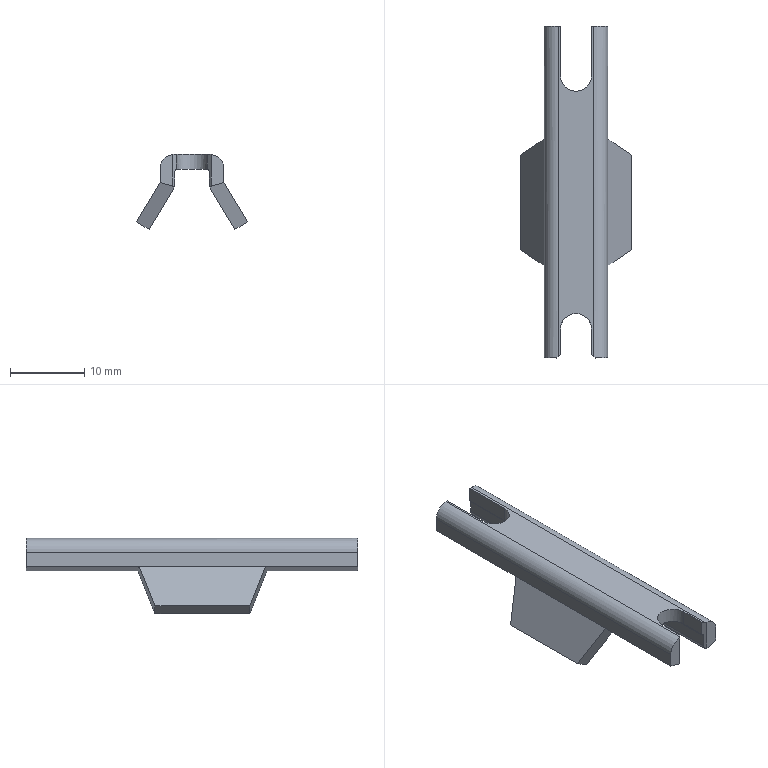Part | STEP file | Y300T_Y3035DB Front Plate_3 | 1 solid | 38 faces | box 14.986 x 44.8 x 10.145 mm | volume 1347 mm3 | plane 30 | cylinder 8 | commonest cylinder face diameters 0.6 x2 3.2 x2 3.8 x2 4.2 x2
STEP:
#1=CARTESIAN_POINT('',(-2.1,23.8,-2.017));
#2=VERTEX_POINT('',#1);
#3=CARTESIAN_POINT('',(-2.1,23.8,0.));
#4=VERTEX_POINT('',#3);
#5=CARTESIAN_POINT('',(-2.1,23.8,-10.145));
#6=DIRECTION('',(0.,0.,1.));
#7=VECTOR('',#6,1000.);
#8=LINE('',#5,#7);
#9=EDGE_CURVE('',#2,#4,#8,.T.);
#10=ORIENTED_EDGE('',*,*,#9,.F.);
#11=CARTESIAN_POINT('',(-2.3,23.8,-2.3));
#12=VERTEX_POINT('',#11);
#13=CARTESIAN_POINT('',(-2.,23.8,-2.3));
#14=DIRECTION('',(0.,1.,0.));
#15=DIRECTION('',(0.,0.,1.));
#16=AXIS2_PLACEMENT_3D('',#13,#14,#15);
#17=CIRCLE('',#16,0.3);
#18=EDGE_CURVE('',#12,#2,#17,.T.);
#19=ORIENTED_EDGE('',*,*,#18,.F.);
#20=CARTESIAN_POINT('',(-2.3,23.8,-3.911));
#21=VERTEX_POINT('',#20);
#22=CARTESIAN_POINT('',(-2.3,23.8,-4.355));
#23=DIRECTION('',(0.,0.,1.));
#24=VECTOR('',#23,1000.);
#25=LINE('',#22,#24);
#26=EDGE_CURVE('',#21,#12,#25,.T.);
#27=ORIENTED_EDGE('',*,*,#26,.F.);
#28=CARTESIAN_POINT('',(-2.363,23.8,-4.355));
#29=VERTEX_POINT('',#28);
#30=CARTESIAN_POINT('',(-3.9,23.8,-3.911));
#31=DIRECTION('',(0.,-1.,0.));
#32=DIRECTION('',(0.,0.,1.));
#33=AXIS2_PLACEMENT_3D('',#30,#31,#32);
#34=CIRCLE('',#33,1.6);
#35=EDGE_CURVE('',#29,#21,#34,.T.);
#36=ORIENTED_EDGE('',*,*,#35,.F.);
#37=CARTESIAN_POINT('',(-4.3,23.8,-3.8));
#38=VERTEX_POINT('',#37);
#39=CARTESIAN_POINT('',(-1.334,23.8,-4.651));
#40=DIRECTION('',(0.9613,0.,-0.2756));
#41=VECTOR('',#40,1000.);
#42=LINE('',#39,#41);
#43=EDGE_CURVE('',#38,#29,#42,.T.);
#44=ORIENTED_EDGE('',*,*,#43,.F.);
#45=CARTESIAN_POINT('',(-4.3,23.8,-1.9));
#46=VERTEX_POINT('',#45);
#47=CARTESIAN_POINT('',(-4.3,23.8,0.));
#48=DIRECTION('',(0.,0.,-1.));
#49=VECTOR('',#48,1000.);
#50=LINE('',#47,#49);
#51=EDGE_CURVE('',#46,#38,#50,.T.);
#52=ORIENTED_EDGE('',*,*,#51,.F.);
#53=CARTESIAN_POINT('',(-2.4,23.8,0.));
#54=VERTEX_POINT('',#53);
#55=CARTESIAN_POINT('',(-2.4,23.8,-1.9));
#56=DIRECTION('',(0.,-1.,0.));
#57=DIRECTION('',(0.,0.,1.));
#58=AXIS2_PLACEMENT_3D('',#55,#56,#57);
#59=CIRCLE('',#58,1.9);
#60=EDGE_CURVE('',#54,#46,#59,.T.);
#61=ORIENTED_EDGE('',*,*,#60,.F.);
#62=CARTESIAN_POINT('',(0.,23.8,0.));
#63=DIRECTION('',(1.,0.,0.));
#64=VECTOR('',#63,1000.);
#65=LINE('',#62,#64);
#66=EDGE_CURVE('',#54,#4,#65,.T.);
#67=ORIENTED_EDGE('',*,*,#66,.T.);
#68=EDGE_LOOP('',(#10,#19,#27,#36,#44,#52,#61,#67));
#69=FACE_OUTER_BOUND('',#68,.T.);
#70=CARTESIAN_POINT('',(0.,23.8,0.));
#71=DIRECTION('',(0.,1.,0.));
#72=DIRECTION('',(0.,0.,1.));
#73=AXIS2_PLACEMENT_3D('',#70,#71,#72);
#74=PLANE('',#73);
#75=ADVANCED_FACE('',(#69),#74,.T.);
#76=CARTESIAN_POINT('',(-4.3,-21.,-3.8));
#77=VERTEX_POINT('',#76);
#78=CARTESIAN_POINT('',(-2.6,-21.,-4.287));
#79=VERTEX_POINT('',#78);
#80=CARTESIAN_POINT('',(-4.3,-21.,-3.8));
#81=DIRECTION('',(0.9613,0.,-0.2756));
#82=VECTOR('',#81,1000.);
#83=LINE('',#80,#82);
#84=EDGE_CURVE('',#77,#79,#83,.T.);
#85=ORIENTED_EDGE('',*,*,#84,.T.);
#86=CARTESIAN_POINT('',(-2.6,-21.,-0.01056));
#87=VERTEX_POINT('',#86);
#88=CARTESIAN_POINT('',(-2.6,-21.,68.405));
#89=DIRECTION('',(0.,0.,1.));
#90=VECTOR('',#89,1000.);
#91=LINE('',#88,#90);
#92=EDGE_CURVE('',#79,#87,#91,.T.);
#93=ORIENTED_EDGE('',*,*,#92,.T.);
#94=CARTESIAN_POINT('',(-4.3,-21.,-1.9));
#95=VERTEX_POINT('',#94);
#96=CARTESIAN_POINT('',(-2.4,-21.,-1.9));
#97=DIRECTION('',(0.,-1.,0.));
#98=DIRECTION('',(0.,0.,1.));
#99=AXIS2_PLACEMENT_3D('',#96,#97,#98);
#100=CIRCLE('',#99,1.9);
#101=EDGE_CURVE('',#87,#95,#100,.T.);
#102=ORIENTED_EDGE('',*,*,#101,.T.);
#103=CARTESIAN_POINT('',(-4.3,-21.,0.));
#104=DIRECTION('',(0.,0.,1.));
#105=VECTOR('',#104,1000.);
#106=LINE('',#103,#105);
#107=EDGE_CURVE('',#77,#95,#106,.T.);
#108=ORIENTED_EDGE('',*,*,#107,.F.);
#109=EDGE_LOOP('',(#85,#93,#102,#108));
#110=FACE_OUTER_BOUND('',#109,.T.);
#111=CARTESIAN_POINT('',(-7.493,-21.,68.405));
#112=DIRECTION('',(0.,1.,0.));
#113=DIRECTION('',(0.,0.,1.));
#114=AXIS2_PLACEMENT_3D('',#111,#112,#113);
#115=PLANE('',#114);
#116=ADVANCED_FACE('',(#110),#115,.F.);
#117=CARTESIAN_POINT('',(7.493,6.4,-9.114));
#118=VERTEX_POINT('',#117);
#119=CARTESIAN_POINT('',(4.3,8.535,-3.8));
#120=VERTEX_POINT('',#119);
#121=CARTESIAN_POINT('',(7.493,6.4,-9.114));
#122=DIRECTION('',(-0.487,0.3256,0.8105));
#123=VECTOR('',#122,1000.);
#124=LINE('',#121,#123);
#125=EDGE_CURVE('',#118,#120,#124,.T.);
#126=ORIENTED_EDGE('',*,*,#125,.T.);
#127=CARTESIAN_POINT('',(4.3,-8.535,-3.8));
#128=VERTEX_POINT('',#127);
#129=CARTESIAN_POINT('',(4.3,23.8,-3.8));
#130=DIRECTION('',(0.,-1.,0.));
#131=VECTOR('',#130,1000.);
#132=LINE('',#129,#131);
#133=EDGE_CURVE('',#120,#128,#132,.T.);
#134=ORIENTED_EDGE('',*,*,#133,.T.);
#135=CARTESIAN_POINT('',(7.493,-6.4,-9.114));
#136=VERTEX_POINT('',#135);
#137=CARTESIAN_POINT('',(7.493,-6.4,-9.114));
#138=DIRECTION('',(-0.487,-0.3256,0.8105));
#139=VECTOR('',#138,1000.);
#140=LINE('',#137,#139);
#141=EDGE_CURVE('',#136,#128,#140,.T.);
#142=ORIENTED_EDGE('',*,*,#141,.F.);
#143=CARTESIAN_POINT('',(7.493,23.8,-9.114));
#144=DIRECTION('',(0.,-1.,0.));
#145=VECTOR('',#144,1000.);
#146=LINE('',#143,#145);
#147=EDGE_CURVE('',#118,#136,#146,.T.);
#148=ORIENTED_EDGE('',*,*,#147,.F.);
#149=EDGE_LOOP('',(#126,#134,#142,#148));
#150=FACE_OUTER_BOUND('',#149,.T.);
#151=CARTESIAN_POINT('',(4.3,23.8,-3.8));
#152=DIRECTION('',(-0.8572,0.,-0.515));
#153=DIRECTION('',(-0.515,0.,0.8572));
#154=AXIS2_PLACEMENT_3D('',#151,#152,#153);
#155=PLANE('',#154);
#156=ADVANCED_FACE('',(#150),#155,.F.);
#157=CARTESIAN_POINT('',(5.779,6.4,-10.145));
#158=VERTEX_POINT('',#157);
#159=CARTESIAN_POINT('',(-13.936,6.4,-21.99));
#160=DIRECTION('',(0.8572,0.,0.515));
#161=VECTOR('',#160,1000.);
#162=LINE('',#159,#161);
#163=EDGE_CURVE('',#158,#118,#162,.T.);
#164=ORIENTED_EDGE('',*,*,#163,.T.);
#165=ORIENTED_EDGE('',*,*,#147,.T.);
#166=CARTESIAN_POINT('',(5.779,-6.4,-10.145));
#167=VERTEX_POINT('',#166);
#168=CARTESIAN_POINT('',(-13.936,-6.4,-21.99));
#169=DIRECTION('',(0.8572,0.,0.515));
#170=VECTOR('',#169,1000.);
#171=LINE('',#168,#170);
#172=EDGE_CURVE('',#167,#136,#171,.T.);
#173=ORIENTED_EDGE('',*,*,#172,.F.);
#174=CARTESIAN_POINT('',(5.779,23.8,-10.145));
#175=DIRECTION('',(0.,-1.,0.));
#176=VECTOR('',#175,1000.);
#177=LINE('',#174,#176);
#178=EDGE_CURVE('',#158,#167,#177,.T.);
#179=ORIENTED_EDGE('',*,*,#178,.F.);
#180=EDGE_LOOP('',(#164,#165,#173,#179));
#181=FACE_OUTER_BOUND('',#180,.T.);
#182=CARTESIAN_POINT('',(7.493,23.8,-9.114));
#183=DIRECTION('',(-0.515,0.,0.8572));
#184=DIRECTION('',(0.8572,0.,0.515));
#185=AXIS2_PLACEMENT_3D('',#182,#183,#184);
#186=PLANE('',#185);
#187=ADVANCED_FACE('',(#181),#186,.F.);
#188=ORIENTED_EDGE('',*,*,#178,.T.);
#189=CARTESIAN_POINT('',(2.529,-8.573,-4.735));
#190=VERTEX_POINT('',#189);
#191=CARTESIAN_POINT('',(5.779,-6.4,-10.145));
#192=DIRECTION('',(0.487,0.3256,-0.8105));
#193=VECTOR('',#192,1000.);
#194=LINE('',#191,#193);
#195=EDGE_CURVE('',#190,#167,#194,.T.);
#196=ORIENTED_EDGE('',*,*,#195,.F.);
#197=CARTESIAN_POINT('',(2.529,8.573,-4.735));
#198=VERTEX_POINT('',#197);
#199=CARTESIAN_POINT('',(2.529,23.8,-4.735));
#200=DIRECTION('',(0.,1.,0.));
#201=VECTOR('',#200,1000.);
#202=LINE('',#199,#201);
#203=EDGE_CURVE('',#190,#198,#202,.T.);
#204=ORIENTED_EDGE('',*,*,#203,.T.);
#205=CARTESIAN_POINT('',(5.779,6.4,-10.145));
#206=DIRECTION('',(0.487,-0.3256,-0.8105));
#207=VECTOR('',#206,1000.);
#208=LINE('',#205,#207);
#209=EDGE_CURVE('',#198,#158,#208,.T.);
#210=ORIENTED_EDGE('',*,*,#209,.T.);
#211=EDGE_LOOP('',(#188,#196,#204,#210));
#212=FACE_OUTER_BOUND('',#211,.T.);
#213=CARTESIAN_POINT('',(5.779,23.8,-10.145));
#214=DIRECTION('',(0.8572,0.,0.515));
#215=DIRECTION('',(0.515,0.,-0.8572));
#216=AXIS2_PLACEMENT_3D('',#213,#214,#215);
#217=PLANE('',#216);
#218=ADVANCED_FACE('',(#212),#217,.F.);
#219=CARTESIAN_POINT('',(2.1,23.8,-2.017));
#220=VERTEX_POINT('',#219);
#221=CARTESIAN_POINT('',(2.1,23.8,0.));
#222=VERTEX_POINT('',#221);
#223=CARTESIAN_POINT('',(2.1,23.8,-10.145));
#224=DIRECTION('',(0.,0.,1.));
#225=VECTOR('',#224,1000.);
#226=LINE('',#223,#225);
#227=EDGE_CURVE('',#220,#222,#226,.T.);
#228=ORIENTED_EDGE('',*,*,#227,.T.);
#229=CARTESIAN_POINT('',(2.4,23.8,0.));
#230=VERTEX_POINT('',#229);
#231=CARTESIAN_POINT('',(0.,23.8,0.));
#232=DIRECTION('',(1.,0.,0.));
#233=VECTOR('',#232,1000.);
#234=LINE('',#231,#233);
#235=EDGE_CURVE('',#222,#230,#234,.T.);
#236=ORIENTED_EDGE('',*,*,#235,.T.);
#237=CARTESIAN_POINT('',(4.3,23.8,-1.9));
#238=VERTEX_POINT('',#237);
#239=CARTESIAN_POINT('',(2.4,23.8,-1.9));
#240=DIRECTION('',(0.,1.,0.));
#241=DIRECTION('',(0.,0.,1.));
#242=AXIS2_PLACEMENT_3D('',#239,#240,#241);
#243=CIRCLE('',#242,1.9);
#244=EDGE_CURVE('',#230,#238,#243,.T.);
#245=ORIENTED_EDGE('',*,*,#244,.T.);
#246=CARTESIAN_POINT('',(4.3,23.8,-3.8));
#247=VERTEX_POINT('',#246);
#248=CARTESIAN_POINT('',(4.3,23.8,0.));
#249=DIRECTION('',(0.,0.,-1.));
#250=VECTOR('',#249,1000.);
#251=LINE('',#248,#250);
#252=EDGE_CURVE('',#238,#247,#251,.T.);
#253=ORIENTED_EDGE('',*,*,#252,.T.);
#254=CARTESIAN_POINT('',(2.363,23.8,-4.355));
#255=VERTEX_POINT('',#254);
#256=CARTESIAN_POINT('',(1.334,23.8,-4.651));
#257=DIRECTION('',(-0.9613,0.,-0.2756));
#258=VECTOR('',#257,1000.);
#259=LINE('',#256,#258);
#260=EDGE_CURVE('',#247,#255,#259,.T.);
#261=ORIENTED_EDGE('',*,*,#260,.T.);
#262=CARTESIAN_POINT('',(2.3,23.8,-3.911));
#263=VERTEX_POINT('',#262);
#264=CARTESIAN_POINT('',(3.9,23.8,-3.911));
#265=DIRECTION('',(0.,1.,0.));
#266=DIRECTION('',(0.,0.,1.));
#267=AXIS2_PLACEMENT_3D('',#264,#265,#266);
#268=CIRCLE('',#267,1.6);
#269=EDGE_CURVE('',#255,#263,#268,.T.);
#270=ORIENTED_EDGE('',*,*,#269,.T.);
#271=CARTESIAN_POINT('',(2.3,23.8,-2.3));
#272=VERTEX_POINT('',#271);
#273=CARTESIAN_POINT('',(2.3,23.8,-4.355));
#274=DIRECTION('',(0.,0.,1.));
#275=VECTOR('',#274,1000.);
#276=LINE('',#273,#275);
#277=EDGE_CURVE('',#263,#272,#276,.T.);
#278=ORIENTED_EDGE('',*,*,#277,.T.);
#279=CARTESIAN_POINT('',(2.,23.8,-2.3));
#280=DIRECTION('',(0.,-1.,0.));
#281=DIRECTION('',(0.,0.,1.));
#282=AXIS2_PLACEMENT_3D('',#279,#280,#281);
#283=CIRCLE('',#282,0.3);
#284=EDGE_CURVE('',#272,#220,#283,.T.);
#285=ORIENTED_EDGE('',*,*,#284,.T.);
#286=EDGE_LOOP('',(#228,#236,#245,#253,#261,#270,#278,#285));
#287=FACE_OUTER_BOUND('',#286,.T.);
#288=CARTESIAN_POINT('',(0.,23.8,0.));
#289=DIRECTION('',(0.,1.,0.));
#290=DIRECTION('',(0.,0.,1.));
#291=AXIS2_PLACEMENT_3D('',#288,#289,#290);
#292=PLANE('',#291);
#293=ADVANCED_FACE('',(#287),#292,.T.);
#294=CARTESIAN_POINT('',(-2.4,-20.8,0.));
#295=VERTEX_POINT('',#294);
#296=CARTESIAN_POINT('',(-2.4,23.8,0.));
#297=DIRECTION('',(0.,1.,0.));
#298=VECTOR('',#297,1000.);
#299=LINE('',#296,#298);
#300=EDGE_CURVE('',#295,#54,#299,.T.);
#301=ORIENTED_EDGE('',*,*,#300,.F.);
#302=CARTESIAN_POINT('',(-2.1,-20.5,0.));
#303=VERTEX_POINT('',#302);
#304=CARTESIAN_POINT('',(-2.6,-21.,0.));
#305=DIRECTION('',(0.7071,0.7071,0.));
#306=VECTOR('',#305,1000.);
#307=LINE('',#304,#306);
#308=EDGE_CURVE('',#295,#303,#307,.T.);
#309=ORIENTED_EDGE('',*,*,#308,.T.);
#310=CARTESIAN_POINT('',(-2.1,-17.1,0.));
#311=VERTEX_POINT('',#310);
#312=CARTESIAN_POINT('',(-2.1,-21.,0.));
#313=DIRECTION('',(0.,-1.,0.));
#314=VECTOR('',#313,1000.);
#315=LINE('',#312,#314);
#316=EDGE_CURVE('',#311,#303,#315,.T.);
#317=ORIENTED_EDGE('',*,*,#316,.F.);
#318=CARTESIAN_POINT('',(2.1,-17.1,0.));
#319=VERTEX_POINT('',#318);
#320=CARTESIAN_POINT('',(0.,-17.1,0.));
#321=DIRECTION('',(0.,0.,1.));
#322=DIRECTION('',(-1.,0.,0.));
#323=AXIS2_PLACEMENT_3D('',#320,#321,#322);
#324=CIRCLE('',#323,2.1);
#325=EDGE_CURVE('',#319,#311,#324,.T.);
#326=ORIENTED_EDGE('',*,*,#325,.F.);
#327=CARTESIAN_POINT('',(2.1,-20.5,0.));
#328=VERTEX_POINT('',#327);
#329=CARTESIAN_POINT('',(2.1,-21.,0.));
#330=DIRECTION('',(0.,1.,0.));
#331=VECTOR('',#330,1000.);
#332=LINE('',#329,#331);
#333=EDGE_CURVE('',#328,#319,#332,.T.);
#334=ORIENTED_EDGE('',*,*,#333,.F.);
#335=CARTESIAN_POINT('',(2.4,-20.8,0.));
#336=VERTEX_POINT('',#335);
#337=CARTESIAN_POINT('',(2.6,-21.,0.));
#338=DIRECTION('',(0.7071,-0.7071,0.));
#339=VECTOR('',#338,1000.);
#340=LINE('',#337,#339);
#341=EDGE_CURVE('',#328,#336,#340,.T.);
#342=ORIENTED_EDGE('',*,*,#341,.T.);
#343=CARTESIAN_POINT('',(2.4,23.8,0.));
#344=DIRECTION('',(0.,1.,0.));
#345=VECTOR('',#344,1000.);
#346=LINE('',#343,#345);
#347=EDGE_CURVE('',#336,#230,#346,.T.);
#348=ORIENTED_EDGE('',*,*,#347,.T.);
#349=ORIENTED_EDGE('',*,*,#235,.F.);
#350=CARTESIAN_POINT('',(2.1,17.1,0.));
#351=VERTEX_POINT('',#350);
#352=CARTESIAN_POINT('',(2.1,23.8,0.));
#353=DIRECTION('',(0.,1.,0.));
#354=VECTOR('',#353,1000.);
#355=LINE('',#352,#354);
#356=EDGE_CURVE('',#351,#222,#355,.T.);
#357=ORIENTED_EDGE('',*,*,#356,.F.);
#358=CARTESIAN_POINT('',(-2.1,17.1,0.));
#359=VERTEX_POINT('',#358);
#360=CARTESIAN_POINT('',(0.,17.1,0.));
#361=DIRECTION('',(0.,0.,1.));
#362=DIRECTION('',(1.,0.,0.));
#363=AXIS2_PLACEMENT_3D('',#360,#361,#362);
#364=CIRCLE('',#363,2.1);
#365=EDGE_CURVE('',#359,#351,#364,.T.);
#366=ORIENTED_EDGE('',*,*,#365,.F.);
#367=CARTESIAN_POINT('',(-2.1,23.8,0.));
#368=DIRECTION('',(0.,-1.,0.));
#369=VECTOR('',#368,1000.);
#370=LINE('',#367,#369);
#371=EDGE_CURVE('',#4,#359,#370,.T.);
#372=ORIENTED_EDGE('',*,*,#371,.F.);
#373=ORIENTED_EDGE('',*,*,#66,.F.);
#374=EDGE_LOOP('',(#301,#309,#317,#326,#334,#342,#348,#349,#357,#366,#372,#373));
#375=FACE_OUTER_BOUND('',#374,.T.);
#376=CARTESIAN_POINT('',(0.,23.8,0.));
#377=DIRECTION('',(0.,0.,-1.));
#378=DIRECTION('',(-1.,0.,0.));
#379=AXIS2_PLACEMENT_3D('',#376,#377,#378);
#380=PLANE('',#379);
#381=ADVANCED_FACE('',(#375),#380,.F.);
#382=CARTESIAN_POINT('',(4.3,-21.,-1.9));
#383=VERTEX_POINT('',#382);
#384=CARTESIAN_POINT('',(4.3,23.8,-1.9));
#385=DIRECTION('',(0.,-1.,0.));
#386=VECTOR('',#385,1000.);
#387=LINE('',#384,#386);
#388=EDGE_CURVE('',#238,#383,#387,.T.);
#389=ORIENTED_EDGE('',*,*,#388,.T.);
#390=CARTESIAN_POINT('',(4.3,-21.,-3.8));
#391=VERTEX_POINT('',#390);
#392=CARTESIAN_POINT('',(4.3,-21.,0.));
#393=DIRECTION('',(0.,0.,-1.));
#394=VECTOR('',#393,1000.);
#395=LINE('',#392,#394);
#396=EDGE_CURVE('',#383,#391,#395,.T.);
#397=ORIENTED_EDGE('',*,*,#396,.T.);
#398=CARTESIAN_POINT('',(4.3,-23.8,-3.8));
#399=DIRECTION('',(0.,1.,0.));
#400=VECTOR('',#399,1000.);
#401=LINE('',#398,#400);
#402=EDGE_CURVE('',#391,#128,#401,.T.);
#403=ORIENTED_EDGE('',*,*,#402,.T.);
#404=ORIENTED_EDGE('',*,*,#133,.F.);
#405=CARTESIAN_POINT('',(4.3,23.8,-3.8));
#406=DIRECTION('',(0.,-1.,0.));
#407=VECTOR('',#406,1000.);
#408=LINE('',#405,#407);
#409=EDGE_CURVE('',#247,#120,#408,.T.);
#410=ORIENTED_EDGE('',*,*,#409,.F.);
#411=ORIENTED_EDGE('',*,*,#252,.F.);
#412=EDGE_LOOP('',(#389,#397,#403,#404,#410,#411));
#413=FACE_OUTER_BOUND('',#412,.T.);
#414=CARTESIAN_POINT('',(4.3,23.8,0.));
#415=DIRECTION('',(-1.,0.,0.));
#416=DIRECTION('',(0.,0.,1.));
#417=AXIS2_PLACEMENT_3D('',#414,#415,#416);
#418=PLANE('',#417);
#419=ADVANCED_FACE('',(#413),#418,.F.);
#420=CARTESIAN_POINT('',(2.3,-20.7,-3.911));
#421=VERTEX_POINT('',#420);
#422=CARTESIAN_POINT('',(2.3,23.8,-3.911));
#423=DIRECTION('',(0.,-1.,0.));
#424=VECTOR('',#423,1000.);
#425=LINE('',#422,#424);
#426=EDGE_CURVE('',#263,#421,#425,.T.);
#427=ORIENTED_EDGE('',*,*,#426,.T.);
#428=CARTESIAN_POINT('',(2.3,-20.7,-2.3));
#429=VERTEX_POINT('',#428);
#430=CARTESIAN_POINT('',(2.3,-20.7,68.405));
#431=DIRECTION('',(0.,0.,1.));
#432=VECTOR('',#431,1000.);
#433=LINE('',#430,#432);
#434=EDGE_CURVE('',#421,#429,#433,.T.);
#435=ORIENTED_EDGE('',*,*,#434,.T.);
#436=CARTESIAN_POINT('',(2.3,23.8,-2.3));
#437=DIRECTION('',(0.,1.,0.));
#438=VECTOR('',#437,1000.);
#439=LINE('',#436,#438);
#440=EDGE_CURVE('',#429,#272,#439,.T.);
#441=ORIENTED_EDGE('',*,*,#440,.T.);
#442=ORIENTED_EDGE('',*,*,#277,.F.);
#443=EDGE_LOOP('',(#427,#435,#441,#442));
#444=FACE_OUTER_BOUND('',#443,.T.);
#445=CARTESIAN_POINT('',(2.3,23.8,-4.355));
#446=DIRECTION('',(1.,0.,0.));
#447=DIRECTION('',(0.,0.,-1.));
#448=AXIS2_PLACEMENT_3D('',#445,#446,#447);
#449=PLANE('',#448);
#450=ADVANCED_FACE('',(#444),#449,.F.);
#451=CARTESIAN_POINT('',(-2.,16.46,-2.));
#452=VERTEX_POINT('',#451);
#453=CARTESIAN_POINT('',(-2.,-16.46,-2.));
#454=VERTEX_POINT('',#453);
#455=CARTESIAN_POINT('',(-2.,0.,-2.));
#456=DIRECTION('',(0.,-1.,0.));
#457=VECTOR('',#456,1000.);
#458=LINE('',#455,#457);
#459=EDGE_CURVE('',#452,#454,#458,.T.);
#460=ORIENTED_EDGE('',*,*,#459,.F.);
#461=CARTESIAN_POINT('',(2.,16.46,-2.));
#462=VERTEX_POINT('',#461);
#463=CARTESIAN_POINT('',(0.,17.1,-2.));
#464=DIRECTION('',(0.,0.,1.));
#465=DIRECTION('',(1.,0.,0.));
#466=AXIS2_PLACEMENT_3D('',#463,#464,#465);
#467=CIRCLE('',#466,2.1);
#468=EDGE_CURVE('',#452,#462,#467,.T.);
#469=ORIENTED_EDGE('',*,*,#468,.T.);
#470=CARTESIAN_POINT('',(2.,-16.46,-2.));
#471=VERTEX_POINT('',#470);
#472=CARTESIAN_POINT('',(2.,0.,-2.));
#473=DIRECTION('',(0.,-1.,0.));
#474=VECTOR('',#473,1000.);
#475=LINE('',#472,#474);
#476=EDGE_CURVE('',#462,#471,#475,.T.);
#477=ORIENTED_EDGE('',*,*,#476,.T.);
#478=CARTESIAN_POINT('',(0.,-17.1,-2.));
#479=DIRECTION('',(0.,0.,1.));
#480=DIRECTION('',(1.,0.,0.));
#481=AXIS2_PLACEMENT_3D('',#478,#479,#480);
#482=CIRCLE('',#481,2.1);
#483=EDGE_CURVE('',#471,#454,#482,.T.);
#484=ORIENTED_EDGE('',*,*,#483,.T.);
#485=EDGE_LOOP('',(#460,#469,#477,#484));
#486=FACE_OUTER_BOUND('',#485,.T.);
#487=CARTESIAN_POINT('',(2.3,23.8,-2.));
#488=DIRECTION('',(0.,0.,1.));
#489=DIRECTION('',(1.,0.,0.));
#490=AXIS2_PLACEMENT_3D('',#487,#488,#489);
#491=PLANE('',#490);
#492=ADVANCED_FACE('',(#486),#491,.F.);
#493=ORIENTED_EDGE('',*,*,#209,.F.);
#494=CARTESIAN_POINT('',(2.363,8.714,-4.355));
#495=VERTEX_POINT('',#494);
#496=CARTESIAN_POINT('',(2.529,8.573,-4.735));
#497=CARTESIAN_POINT('',(2.457,8.621,-4.616));
#498=CARTESIAN_POINT('',(2.402,8.668,-4.489));
#499=CARTESIAN_POINT('',(2.363,8.714,-4.355));
#500=(BOUNDED_CURVE()B_SPLINE_CURVE(3,(#496,#497,#498,#499),.UNSPECIFIED.,.F.,.F.)B_SPLINE_CURVE_WITH_KNOTS((4,4),(1.571,1.83),.UNSPECIFIED.)CURVE()GEOMETRIC_REPRESENTATION_ITEM()RATIONAL_B_SPLINE_CURVE((1.,0.9944,0.9944,1.))REPRESENTATION_ITEM(''));
#501=EDGE_CURVE('',#198,#495,#500,.T.);
#502=ORIENTED_EDGE('',*,*,#501,.T.);
#503=CARTESIAN_POINT('',(-17.018,10.511,-9.913));
#504=DIRECTION('',(-0.9575,0.08877,-0.2745));
#505=VECTOR('',#504,1000.);
#506=LINE('',#503,#505);
#507=EDGE_CURVE('',#120,#495,#506,.T.);
#508=ORIENTED_EDGE('',*,*,#507,.F.);
#509=ORIENTED_EDGE('',*,*,#125,.F.);
#510=ORIENTED_EDGE('',*,*,#163,.F.);
#511=EDGE_LOOP('',(#493,#502,#508,#509,#510));
#512=FACE_OUTER_BOUND('',#511,.T.);
#513=CARTESIAN_POINT('',(-13.936,6.4,-21.99));
#514=DIRECTION('',(0.1677,0.9455,-0.2791));
#515=DIRECTION('',(0.,0.2831,0.9591));
#516=AXIS2_PLACEMENT_3D('',#513,#514,#515);
#517=PLANE('',#516);
#518=ADVANCED_FACE('',(#512),#517,.T.);
#519=ORIENTED_EDGE('',*,*,#507,.T.);
#520=CARTESIAN_POINT('',(2.363,8.714,-4.355));
#521=DIRECTION('',(0.,1.,0.));
#522=VECTOR('',#521,1000.);
#523=LINE('',#520,#522);
#524=EDGE_CURVE('',#495,#255,#523,.T.);
#525=ORIENTED_EDGE('',*,*,#524,.T.);
#526=ORIENTED_EDGE('',*,*,#260,.F.);
#527=ORIENTED_EDGE('',*,*,#409,.T.);
#528=EDGE_LOOP('',(#519,#525,#526,#527));
#529=FACE_OUTER_BOUND('',#528,.T.);
#530=CARTESIAN_POINT('',(4.3,0.,-3.8));
#531=DIRECTION('',(0.2756,0.,-0.9613));
#532=DIRECTION('',(-0.9613,0.,-0.2756));
#533=AXIS2_PLACEMENT_3D('',#530,#531,#532);
#534=PLANE('',#533);
#535=ADVANCED_FACE('',(#529),#534,.T.);
#536=ORIENTED_EDGE('',*,*,#347,.F.);
#537=CARTESIAN_POINT('',(2.6,-21.,-0.01056));
#538=VERTEX_POINT('',#537);
#539=CARTESIAN_POINT('',(2.4,-20.8,0.));
#540=CARTESIAN_POINT('',(2.467,-20.867,0.));
#541=CARTESIAN_POINT('',(2.534,-20.934,-0.003522));
#542=CARTESIAN_POINT('',(2.6,-21.,-0.01056));
#543=(BOUNDED_CURVE()B_SPLINE_CURVE(3,(#539,#540,#541,#542),.UNSPECIFIED.,.F.,.F.)B_SPLINE_CURVE_WITH_KNOTS((4,4),(4.712,4.818),.UNSPECIFIED.)CURVE()GEOMETRIC_REPRESENTATION_ITEM()RATIONAL_B_SPLINE_CURVE((1.,0.9991,0.9991,1.))REPRESENTATION_ITEM(''));
#544=EDGE_CURVE('',#336,#538,#543,.T.);
#545=ORIENTED_EDGE('',*,*,#544,.T.);
#546=CARTESIAN_POINT('',(2.4,-21.,-1.9));
#547=DIRECTION('',(0.,-1.,0.));
#548=DIRECTION('',(0.,0.,1.));
#549=AXIS2_PLACEMENT_3D('',#546,#547,#548);
#550=CIRCLE('',#549,1.9);
#551=EDGE_CURVE('',#383,#538,#550,.T.);
#552=ORIENTED_EDGE('',*,*,#551,.F.);
#553=ORIENTED_EDGE('',*,*,#388,.F.);
#554=ORIENTED_EDGE('',*,*,#244,.F.);
#555=EDGE_LOOP('',(#536,#545,#552,#553,#554));
#556=FACE_OUTER_BOUND('',#555,.T.);
#557=CARTESIAN_POINT('',(2.4,23.8,-1.9));
#558=DIRECTION('',(0.,-1.,0.));
#559=DIRECTION('',(0.,0.,-1.));
#560=AXIS2_PLACEMENT_3D('',#557,#558,#559);
#561=CYLINDRICAL_SURFACE('',#560,1.9);
#562=ADVANCED_FACE('',(#556),#561,.T.);
#563=ORIENTED_EDGE('',*,*,#440,.F.);
#564=CARTESIAN_POINT('',(2.1,-20.5,-2.017));
#565=VERTEX_POINT('',#564);
#566=CARTESIAN_POINT('',(2.3,-20.7,-2.3));
#567=CARTESIAN_POINT('',(2.3,-20.7,-2.168));
#568=CARTESIAN_POINT('',(2.224,-20.624,-2.061));
#569=CARTESIAN_POINT('',(2.1,-20.5,-2.017));
#570=(BOUNDED_CURVE()B_SPLINE_CURVE(3,(#566,#567,#568,#569),.UNSPECIFIED.,.F.,.F.)B_SPLINE_CURVE_WITH_KNOTS((4,4),(3.142,4.373),.UNSPECIFIED.)CURVE()GEOMETRIC_REPRESENTATION_ITEM()RATIONAL_B_SPLINE_CURVE((1.,0.8777,0.8777,1.))REPRESENTATION_ITEM(''));
#571=EDGE_CURVE('',#429,#565,#570,.T.);
#572=ORIENTED_EDGE('',*,*,#571,.T.);
#573=CARTESIAN_POINT('',(2.1,-17.1,-2.017));
#574=VERTEX_POINT('',#573);
#575=CARTESIAN_POINT('',(2.1,23.8,-2.017));
#576=DIRECTION('',(0.,1.,0.));
#577=VECTOR('',#576,1000.);
#578=LINE('',#575,#577);
#579=EDGE_CURVE('',#565,#574,#578,.T.);
#580=ORIENTED_EDGE('',*,*,#579,.T.);
#581=CARTESIAN_POINT('',(2.1,-17.1,-2.017));
#582=CARTESIAN_POINT('',(2.1,-16.882,-2.017));
#583=CARTESIAN_POINT('',(2.067,-16.667,-2.));
#584=CARTESIAN_POINT('',(2.,-16.46,-2.));
#585=B_SPLINE_CURVE_WITH_KNOTS('',3,(#581,#582,#583,#584),.UNSPECIFIED.,.F.,.F.,(4,4),(0.0006066,0.001255),.UNSPECIFIED.);
#586=EDGE_CURVE('',#574,#471,#585,.T.);
#587=ORIENTED_EDGE('',*,*,#586,.T.);
#588=ORIENTED_EDGE('',*,*,#476,.F.);
#589=CARTESIAN_POINT('',(2.1,17.1,-2.017));
#590=VERTEX_POINT('',#589);
#591=CARTESIAN_POINT('',(2.,16.46,-2.));
#592=CARTESIAN_POINT('',(2.033,16.564,-2.));
#593=CARTESIAN_POINT('',(2.058,16.67,-2.005));
#594=CARTESIAN_POINT('',(2.092,16.883,-2.014));
#595=CARTESIAN_POINT('',(2.1,16.991,-2.017));
#596=CARTESIAN_POINT('',(2.1,17.1,-2.017));
#597=B_SPLINE_CURVE_WITH_KNOTS('',3,(#591,#592,#593,#594,#595,#596),.UNSPECIFIED.,.F.,.F.,(4,2,4),(0.002836,0.003161,0.003485),.UNSPECIFIED.);
#598=EDGE_CURVE('',#462,#590,#597,.T.);
#599=ORIENTED_EDGE('',*,*,#598,.T.);
#600=CARTESIAN_POINT('',(2.1,23.8,-2.017));
#601=DIRECTION('',(0.,1.,0.));
#602=VECTOR('',#601,1000.);
#603=LINE('',#600,#602);
#604=EDGE_CURVE('',#590,#220,#603,.T.);
#605=ORIENTED_EDGE('',*,*,#604,.T.);
#606=ORIENTED_EDGE('',*,*,#284,.F.);
#607=EDGE_LOOP('',(#563,#572,#580,#587,#588,#599,#605,#606));
#608=FACE_OUTER_BOUND('',#607,.T.);
#609=CARTESIAN_POINT('',(2.,23.8,-2.3));
#610=DIRECTION('',(0.,1.,0.));
#611=DIRECTION('',(0.,0.,1.));
#612=AXIS2_PLACEMENT_3D('',#609,#610,#611);
#613=CYLINDRICAL_SURFACE('',#612,0.3);
#614=ADVANCED_FACE('',(#608),#613,.F.);
#615=CARTESIAN_POINT('',(2.363,-8.714,-4.355));
#616=VERTEX_POINT('',#615);
#617=CARTESIAN_POINT('',(2.363,-20.763,-4.355));
#618=VERTEX_POINT('',#617);
#619=CARTESIAN_POINT('',(2.363,-8.714,-4.355));
#620=DIRECTION('',(0.,-1.,0.));
#621=VECTOR('',#620,1000.);
#622=LINE('',#619,#621);
#623=EDGE_CURVE('',#616,#618,#622,.T.);
#624=ORIENTED_EDGE('',*,*,#623,.T.);
#625=CARTESIAN_POINT('',(2.363,-20.763,-4.355));
#626=CARTESIAN_POINT('',(2.321,-20.721,-4.211));
#627=CARTESIAN_POINT('',(2.3,-20.7,-4.062));
#628=CARTESIAN_POINT('',(2.3,-20.7,-3.911));
#629=(BOUNDED_CURVE()B_SPLINE_CURVE(3,(#625,#626,#627,#628),.UNSPECIFIED.,.F.,.F.)B_SPLINE_CURVE_WITH_KNOTS((4,4),(2.86,3.142),.UNSPECIFIED.)CURVE()GEOMETRIC_REPRESENTATION_ITEM()RATIONAL_B_SPLINE_CURVE((1.,0.9934,0.9934,1.))REPRESENTATION_ITEM(''));
#630=EDGE_CURVE('',#618,#421,#629,.T.);
#631=ORIENTED_EDGE('',*,*,#630,.T.);
#632=ORIENTED_EDGE('',*,*,#426,.F.);
#633=ORIENTED_EDGE('',*,*,#269,.F.);
#634=ORIENTED_EDGE('',*,*,#524,.F.);
#635=ORIENTED_EDGE('',*,*,#501,.F.);
#636=ORIENTED_EDGE('',*,*,#203,.F.);
#637=CARTESIAN_POINT('',(2.529,-8.573,-4.735));
#638=CARTESIAN_POINT('',(2.457,-8.621,-4.616));
#639=CARTESIAN_POINT('',(2.402,-8.668,-4.489));
#640=CARTESIAN_POINT('',(2.363,-8.714,-4.355));
#641=(BOUNDED_CURVE()B_SPLINE_CURVE(3,(#637,#638,#639,#640),.UNSPECIFIED.,.F.,.F.)B_SPLINE_CURVE_WITH_KNOTS((4,4),(1.571,1.83),.UNSPECIFIED.)CURVE()GEOMETRIC_REPRESENTATION_ITEM()RATIONAL_B_SPLINE_CURVE((1.,0.9944,0.9944,1.))REPRESENTATION_ITEM(''));
#642=EDGE_CURVE('',#190,#616,#641,.T.);
#643=ORIENTED_EDGE('',*,*,#642,.T.);
#644=EDGE_LOOP('',(#624,#631,#632,#633,#634,#635,#636,#643));
#645=FACE_OUTER_BOUND('',#644,.T.);
#646=CARTESIAN_POINT('',(3.9,23.8,-3.911));
#647=DIRECTION('',(0.,-1.,0.));
#648=DIRECTION('',(0.,0.,-1.));
#649=AXIS2_PLACEMENT_3D('',#646,#647,#648);
#650=CYLINDRICAL_SURFACE('',#649,1.6);
#651=ADVANCED_FACE('',(#645),#650,.T.);
#652=CARTESIAN_POINT('',(2.6,-21.,-4.287));
#653=VERTEX_POINT('',#652);
#654=CARTESIAN_POINT('',(4.3,-21.,-3.8));
#655=DIRECTION('',(0.9613,0.,0.2756));
#656=VECTOR('',#655,1000.);
#657=LINE('',#654,#656);
#658=EDGE_CURVE('',#653,#391,#657,.T.);
#659=ORIENTED_EDGE('',*,*,#658,.F.);
#660=CARTESIAN_POINT('',(-6.602,-11.798,-6.926));
#661=DIRECTION('',(-0.693,0.693,-0.1987));
#662=VECTOR('',#661,1000.);
#663=LINE('',#660,#662);
#664=EDGE_CURVE('',#653,#618,#663,.T.);
#665=ORIENTED_EDGE('',*,*,#664,.T.);
#666=ORIENTED_EDGE('',*,*,#623,.F.);
#667=CARTESIAN_POINT('',(-17.018,-10.511,-9.913));
#668=DIRECTION('',(-0.9575,-0.08877,-0.2745));
#669=VECTOR('',#668,1000.);
#670=LINE('',#667,#669);
#671=EDGE_CURVE('',#128,#616,#670,.T.);
#672=ORIENTED_EDGE('',*,*,#671,.F.);
#673=ORIENTED_EDGE('',*,*,#402,.F.);
#674=EDGE_LOOP('',(#659,#665,#666,#672,#673));
#675=FACE_OUTER_BOUND('',#674,.T.);
#676=CARTESIAN_POINT('',(4.3,0.,-3.8));
#677=DIRECTION('',(0.2756,0.,-0.9613));
#678=DIRECTION('',(-0.9613,0.,-0.2756));
#679=AXIS2_PLACEMENT_3D('',#676,#677,#678);
#680=PLANE('',#679);
#681=ADVANCED_FACE('',(#675),#680,.T.);
#682=ORIENTED_EDGE('',*,*,#195,.T.);
#683=ORIENTED_EDGE('',*,*,#172,.T.);
#684=ORIENTED_EDGE('',*,*,#141,.T.);
#685=ORIENTED_EDGE('',*,*,#671,.T.);
#686=ORIENTED_EDGE('',*,*,#642,.F.);
#687=EDGE_LOOP('',(#682,#683,#684,#685,#686));
#688=FACE_OUTER_BOUND('',#687,.T.);
#689=CARTESIAN_POINT('',(-13.936,-6.4,-21.99));
#690=DIRECTION('',(0.1677,-0.9455,-0.2791));
#691=DIRECTION('',(0.,-0.2831,0.9591));
#692=AXIS2_PLACEMENT_3D('',#689,#690,#691);
#693=PLANE('',#692);
#694=ADVANCED_FACE('',(#688),#693,.T.);
#695=CARTESIAN_POINT('',(-7.493,6.4,-9.114));
#696=VERTEX_POINT('',#695);
#697=CARTESIAN_POINT('',(-4.3,8.535,-3.8));
#698=VERTEX_POINT('',#697);
#699=CARTESIAN_POINT('',(-7.493,6.4,-9.114));
#700=DIRECTION('',(0.487,0.3256,0.8105));
#701=VECTOR('',#700,1000.);
#702=LINE('',#699,#701);
#703=EDGE_CURVE('',#696,#698,#702,.T.);
#704=ORIENTED_EDGE('',*,*,#703,.F.);
#705=CARTESIAN_POINT('',(-7.493,-6.4,-9.114));
#706=VERTEX_POINT('',#705);
#707=CARTESIAN_POINT('',(-7.493,23.8,-9.114));
#708=DIRECTION('',(0.,-1.,0.));
#709=VECTOR('',#708,1000.);
#710=LINE('',#707,#709);
#711=EDGE_CURVE('',#696,#706,#710,.T.);
#712=ORIENTED_EDGE('',*,*,#711,.T.);
#713=CARTESIAN_POINT('',(-4.3,-8.535,-3.8));
#714=VERTEX_POINT('',#713);
#715=CARTESIAN_POINT('',(-7.493,-6.4,-9.114));
#716=DIRECTION('',(0.487,-0.3256,0.8105));
#717=VECTOR('',#716,1000.);
#718=LINE('',#715,#717);
#719=EDGE_CURVE('',#706,#714,#718,.T.);
#720=ORIENTED_EDGE('',*,*,#719,.T.);
#721=CARTESIAN_POINT('',(-4.3,23.8,-3.8));
#722=DIRECTION('',(0.,-1.,0.));
#723=VECTOR('',#722,1000.);
#724=LINE('',#721,#723);
#725=EDGE_CURVE('',#698,#714,#724,.T.);
#726=ORIENTED_EDGE('',*,*,#725,.F.);
#727=EDGE_LOOP('',(#704,#712,#720,#726));
#728=FACE_OUTER_BOUND('',#727,.T.);
#729=CARTESIAN_POINT('',(-4.3,23.8,-3.8));
#730=DIRECTION('',(0.8572,0.,-0.515));
#731=DIRECTION('',(0.515,0.,0.8572));
#732=AXIS2_PLACEMENT_3D('',#729,#730,#731);
#733=PLANE('',#732);
#734=ADVANCED_FACE('',(#728),#733,.F.);
#735=CARTESIAN_POINT('',(-5.779,6.4,-10.145));
#736=VERTEX_POINT('',#735);
#737=CARTESIAN_POINT('',(13.936,6.4,-21.99));
#738=DIRECTION('',(-0.8572,0.,0.515));
#739=VECTOR('',#738,1000.);
#740=LINE('',#737,#739);
#741=EDGE_CURVE('',#736,#696,#740,.T.);
#742=ORIENTED_EDGE('',*,*,#741,.F.);
#743=CARTESIAN_POINT('',(-5.779,-6.4,-10.145));
#744=VERTEX_POINT('',#743);
#745=CARTESIAN_POINT('',(-5.779,23.8,-10.145));
#746=DIRECTION('',(0.,-1.,0.));
#747=VECTOR('',#746,1000.);
#748=LINE('',#745,#747);
#749=EDGE_CURVE('',#736,#744,#748,.T.);
#750=ORIENTED_EDGE('',*,*,#749,.T.);
#751=CARTESIAN_POINT('',(13.936,-6.4,-21.99));
#752=DIRECTION('',(-0.8572,0.,0.515));
#753=VECTOR('',#752,1000.);
#754=LINE('',#751,#753);
#755=EDGE_CURVE('',#744,#706,#754,.T.);
#756=ORIENTED_EDGE('',*,*,#755,.T.);
#757=ORIENTED_EDGE('',*,*,#711,.F.);
#758=EDGE_LOOP('',(#742,#750,#756,#757));
#759=FACE_OUTER_BOUND('',#758,.T.);
#760=CARTESIAN_POINT('',(-7.493,23.8,-9.114));
#761=DIRECTION('',(0.515,0.,0.8572));
#762=DIRECTION('',(-0.8572,0.,0.515));
#763=AXIS2_PLACEMENT_3D('',#760,#761,#762);
#764=PLANE('',#763);
#765=ADVANCED_FACE('',(#759),#764,.F.);
#766=ORIENTED_EDGE('',*,*,#749,.F.);
#767=CARTESIAN_POINT('',(-2.529,8.573,-4.735));
#768=VERTEX_POINT('',#767);
#769=CARTESIAN_POINT('',(-5.779,6.4,-10.145));
#770=DIRECTION('',(-0.487,-0.3256,-0.8105));
#771=VECTOR('',#770,1000.);
#772=LINE('',#769,#771);
#773=EDGE_CURVE('',#768,#736,#772,.T.);
#774=ORIENTED_EDGE('',*,*,#773,.F.);
#775=CARTESIAN_POINT('',(-2.529,-8.573,-4.735));
#776=VERTEX_POINT('',#775);
#777=CARTESIAN_POINT('',(-2.529,23.8,-4.735));
#778=DIRECTION('',(0.,1.,0.));
#779=VECTOR('',#778,1000.);
#780=LINE('',#777,#779);
#781=EDGE_CURVE('',#776,#768,#780,.T.);
#782=ORIENTED_EDGE('',*,*,#781,.F.);
#783=CARTESIAN_POINT('',(-5.779,-6.4,-10.145));
#784=DIRECTION('',(-0.487,0.3256,-0.8105));
#785=VECTOR('',#784,1000.);
#786=LINE('',#783,#785);
#787=EDGE_CURVE('',#776,#744,#786,.T.);
#788=ORIENTED_EDGE('',*,*,#787,.T.);
#789=EDGE_LOOP('',(#766,#774,#782,#788));
#790=FACE_OUTER_BOUND('',#789,.T.);
#791=CARTESIAN_POINT('',(-5.779,23.8,-10.145));
#792=DIRECTION('',(-0.8572,0.,0.515));
#793=DIRECTION('',(-0.515,0.,-0.8572));
#794=AXIS2_PLACEMENT_3D('',#791,#792,#793);
#795=PLANE('',#794);
#796=ADVANCED_FACE('',(#790),#795,.F.);
#797=CARTESIAN_POINT('',(-4.3,-23.8,-3.8));
#798=DIRECTION('',(0.,1.,0.));
#799=VECTOR('',#798,1000.);
#800=LINE('',#797,#799);
#801=EDGE_CURVE('',#77,#714,#800,.T.);
#802=ORIENTED_EDGE('',*,*,#801,.F.);
#803=ORIENTED_EDGE('',*,*,#107,.T.);
#804=CARTESIAN_POINT('',(-4.3,23.8,-1.9));
#805=DIRECTION('',(0.,-1.,0.));
#806=VECTOR('',#805,1000.);
#807=LINE('',#804,#806);
#808=EDGE_CURVE('',#46,#95,#807,.T.);
#809=ORIENTED_EDGE('',*,*,#808,.F.);
#810=ORIENTED_EDGE('',*,*,#51,.T.);
#811=CARTESIAN_POINT('',(-4.3,23.8,-3.8));
#812=DIRECTION('',(0.,-1.,0.));
#813=VECTOR('',#812,1000.);
#814=LINE('',#811,#813);
#815=EDGE_CURVE('',#38,#698,#814,.T.);
#816=ORIENTED_EDGE('',*,*,#815,.T.);
#817=ORIENTED_EDGE('',*,*,#725,.T.);
#818=EDGE_LOOP('',(#802,#803,#809,#810,#816,#817));
#819=FACE_OUTER_BOUND('',#818,.T.);
#820=CARTESIAN_POINT('',(-4.3,23.8,0.));
#821=DIRECTION('',(1.,0.,0.));
#822=DIRECTION('',(0.,0.,1.));
#823=AXIS2_PLACEMENT_3D('',#820,#821,#822);
#824=PLANE('',#823);
#825=ADVANCED_FACE('',(#819),#824,.F.);
#826=CARTESIAN_POINT('',(-2.3,-20.7,-2.3));
#827=VERTEX_POINT('',#826);
#828=CARTESIAN_POINT('',(-2.3,23.8,-2.3));
#829=DIRECTION('',(0.,1.,0.));
#830=VECTOR('',#829,1000.);
#831=LINE('',#828,#830);
#832=EDGE_CURVE('',#827,#12,#831,.T.);
#833=ORIENTED_EDGE('',*,*,#832,.F.);
#834=CARTESIAN_POINT('',(-2.3,-20.7,-3.911));
#835=VERTEX_POINT('',#834);
#836=CARTESIAN_POINT('',(-2.3,-20.7,68.405));
#837=DIRECTION('',(0.,0.,-1.));
#838=VECTOR('',#837,1000.);
#839=LINE('',#836,#838);
#840=EDGE_CURVE('',#827,#835,#839,.T.);
#841=ORIENTED_EDGE('',*,*,#840,.T.);
#842=CARTESIAN_POINT('',(-2.3,23.8,-3.911));
#843=DIRECTION('',(0.,-1.,0.));
#844=VECTOR('',#843,1000.);
#845=LINE('',#842,#844);
#846=EDGE_CURVE('',#21,#835,#845,.T.);
#847=ORIENTED_EDGE('',*,*,#846,.F.);
#848=ORIENTED_EDGE('',*,*,#26,.T.);
#849=EDGE_LOOP('',(#833,#841,#847,#848));
#850=FACE_OUTER_BOUND('',#849,.T.);
#851=CARTESIAN_POINT('',(-2.3,23.8,-4.355));
#852=DIRECTION('',(-1.,0.,0.));
#853=DIRECTION('',(0.,0.,-1.));
#854=AXIS2_PLACEMENT_3D('',#851,#852,#853);
#855=PLANE('',#854);
#856=ADVANCED_FACE('',(#850),#855,.F.);
#857=CARTESIAN_POINT('',(-2.363,8.714,-4.355));
#858=VERTEX_POINT('',#857);
#859=CARTESIAN_POINT('',(17.018,10.511,-9.913));
#860=DIRECTION('',(0.9575,0.08877,-0.2745));
#861=VECTOR('',#860,1000.);
#862=LINE('',#859,#861);
#863=EDGE_CURVE('',#698,#858,#862,.T.);
#864=ORIENTED_EDGE('',*,*,#863,.F.);
#865=ORIENTED_EDGE('',*,*,#815,.F.);
#866=ORIENTED_EDGE('',*,*,#43,.T.);
#867=CARTESIAN_POINT('',(-2.363,8.714,-4.355));
#868=DIRECTION('',(0.,1.,0.));
#869=VECTOR('',#868,1000.);
#870=LINE('',#867,#869);
#871=EDGE_CURVE('',#858,#29,#870,.T.);
#872=ORIENTED_EDGE('',*,*,#871,.F.);
#873=EDGE_LOOP('',(#864,#865,#866,#872));
#874=FACE_OUTER_BOUND('',#873,.T.);
#875=CARTESIAN_POINT('',(-4.3,0.,-3.8));
#876=DIRECTION('',(-0.2756,0.,-0.9613));
#877=DIRECTION('',(0.9613,0.,-0.2756));
#878=AXIS2_PLACEMENT_3D('',#875,#876,#877);
#879=PLANE('',#878);
#880=ADVANCED_FACE('',(#874),#879,.T.);
#881=ORIENTED_EDGE('',*,*,#773,.T.);
#882=ORIENTED_EDGE('',*,*,#741,.T.);
#883=ORIENTED_EDGE('',*,*,#703,.T.);
#884=ORIENTED_EDGE('',*,*,#863,.T.);
#885=CARTESIAN_POINT('',(-2.529,8.573,-4.735));
#886=CARTESIAN_POINT('',(-2.457,8.621,-4.616));
#887=CARTESIAN_POINT('',(-2.402,8.668,-4.489));
#888=CARTESIAN_POINT('',(-2.363,8.714,-4.355));
#889=(BOUNDED_CURVE()B_SPLINE_CURVE(3,(#885,#886,#887,#888),.UNSPECIFIED.,.F.,.F.)B_SPLINE_CURVE_WITH_KNOTS((4,4),(1.571,1.83),.UNSPECIFIED.)CURVE()GEOMETRIC_REPRESENTATION_ITEM()RATIONAL_B_SPLINE_CURVE((1.,0.9944,0.9944,1.))REPRESENTATION_ITEM(''));
#890=EDGE_CURVE('',#768,#858,#889,.T.);
#891=ORIENTED_EDGE('',*,*,#890,.F.);
#892=EDGE_LOOP('',(#881,#882,#883,#884,#891));
#893=FACE_OUTER_BOUND('',#892,.T.);
#894=CARTESIAN_POINT('',(13.936,6.4,-21.99));
#895=DIRECTION('',(-0.1677,0.9455,-0.2791));
#896=DIRECTION('',(0.,0.2831,0.9591));
#897=AXIS2_PLACEMENT_3D('',#894,#895,#896);
#898=PLANE('',#897);
#899=ADVANCED_FACE('',(#893),#898,.T.);
#900=ORIENTED_EDGE('',*,*,#101,.F.);
#901=CARTESIAN_POINT('',(-2.6,-21.,-0.01056));
#902=CARTESIAN_POINT('',(-2.534,-20.934,-0.003522));
#903=CARTESIAN_POINT('',(-2.467,-20.867,0.));
#904=CARTESIAN_POINT('',(-2.4,-20.8,0.));
#905=(BOUNDED_CURVE()B_SPLINE_CURVE(3,(#901,#902,#903,#904),.UNSPECIFIED.,.F.,.T.)B_SPLINE_CURVE_WITH_KNOTS((4,4),(1.465,1.571),.UNSPECIFIED.)CURVE()GEOMETRIC_REPRESENTATION_ITEM()RATIONAL_B_SPLINE_CURVE((1.,0.9991,0.9991,1.))REPRESENTATION_ITEM(''));
#906=EDGE_CURVE('',#87,#295,#905,.T.);
#907=ORIENTED_EDGE('',*,*,#906,.T.);
#908=ORIENTED_EDGE('',*,*,#300,.T.);
#909=ORIENTED_EDGE('',*,*,#60,.T.);
#910=ORIENTED_EDGE('',*,*,#808,.T.);
#911=EDGE_LOOP('',(#900,#907,#908,#909,#910));
#912=FACE_OUTER_BOUND('',#911,.T.);
#913=CARTESIAN_POINT('',(-2.4,23.8,-1.9));
#914=DIRECTION('',(0.,-1.,0.));
#915=DIRECTION('',(0.,0.,-1.));
#916=AXIS2_PLACEMENT_3D('',#913,#914,#915);
#917=CYLINDRICAL_SURFACE('',#916,1.9);
#918=ADVANCED_FACE('',(#912),#917,.T.);
#919=CARTESIAN_POINT('',(-2.1,-17.1,-2.017));
#920=VERTEX_POINT('',#919);
#921=CARTESIAN_POINT('',(-2.1,-20.5,-2.017));
#922=VERTEX_POINT('',#921);
#923=CARTESIAN_POINT('',(-2.1,23.8,-2.017));
#924=DIRECTION('',(0.,-1.,0.));
#925=VECTOR('',#924,1000.);
#926=LINE('',#923,#925);
#927=EDGE_CURVE('',#920,#922,#926,.T.);
#928=ORIENTED_EDGE('',*,*,#927,.T.);
#929=CARTESIAN_POINT('',(-2.1,-20.5,-2.017));
#930=CARTESIAN_POINT('',(-2.224,-20.624,-2.061));
#931=CARTESIAN_POINT('',(-2.3,-20.7,-2.168));
#932=CARTESIAN_POINT('',(-2.3,-20.7,-2.3));
#933=(BOUNDED_CURVE()B_SPLINE_CURVE(3,(#929,#930,#931,#932),.UNSPECIFIED.,.F.,.F.)B_SPLINE_CURVE_WITH_KNOTS((4,4),(1.911,3.142),.UNSPECIFIED.)CURVE()GEOMETRIC_REPRESENTATION_ITEM()RATIONAL_B_SPLINE_CURVE((1.,0.8777,0.8777,1.))REPRESENTATION_ITEM(''));
#934=EDGE_CURVE('',#922,#827,#933,.T.);
#935=ORIENTED_EDGE('',*,*,#934,.T.);
#936=ORIENTED_EDGE('',*,*,#832,.T.);
#937=ORIENTED_EDGE('',*,*,#18,.T.);
#938=CARTESIAN_POINT('',(-2.1,17.1,-2.017));
#939=VERTEX_POINT('',#938);
#940=CARTESIAN_POINT('',(-2.1,23.8,-2.017));
#941=DIRECTION('',(0.,-1.,0.));
#942=VECTOR('',#941,1000.);
#943=LINE('',#940,#942);
#944=EDGE_CURVE('',#2,#939,#943,.T.);
#945=ORIENTED_EDGE('',*,*,#944,.T.);
#946=CARTESIAN_POINT('',(-2.1,17.1,-2.017));
#947=CARTESIAN_POINT('',(-2.1,16.882,-2.017));
#948=CARTESIAN_POINT('',(-2.067,16.667,-2.));
#949=CARTESIAN_POINT('',(-2.,16.46,-2.));
#950=B_SPLINE_CURVE_WITH_KNOTS('',3,(#946,#947,#948,#949),.UNSPECIFIED.,.F.,.F.,(4,4),(0.0006066,0.001255),.UNSPECIFIED.);
#951=EDGE_CURVE('',#939,#452,#950,.T.);
#952=ORIENTED_EDGE('',*,*,#951,.T.);
#953=ORIENTED_EDGE('',*,*,#459,.T.);
#954=CARTESIAN_POINT('',(-2.,-16.46,-2.));
#955=CARTESIAN_POINT('',(-2.033,-16.564,-2.));
#956=CARTESIAN_POINT('',(-2.058,-16.67,-2.005));
#957=CARTESIAN_POINT('',(-2.092,-16.883,-2.014));
#958=CARTESIAN_POINT('',(-2.1,-16.991,-2.017));
#959=CARTESIAN_POINT('',(-2.1,-17.1,-2.017));
#960=B_SPLINE_CURVE_WITH_KNOTS('',3,(#954,#955,#956,#957,#958,#959),.UNSPECIFIED.,.F.,.F.,(4,2,4),(0.002836,0.003161,0.003485),.UNSPECIFIED.);
#961=EDGE_CURVE('',#454,#920,#960,.T.);
#962=ORIENTED_EDGE('',*,*,#961,.T.);
#963=EDGE_LOOP('',(#928,#935,#936,#937,#945,#952,#953,#962));
#964=FACE_OUTER_BOUND('',#963,.T.);
#965=CARTESIAN_POINT('',(-2.,23.8,-2.3));
#966=DIRECTION('',(0.,1.,0.));
#967=DIRECTION('',(0.,0.,1.));
#968=AXIS2_PLACEMENT_3D('',#965,#966,#967);
#969=CYLINDRICAL_SURFACE('',#968,0.3);
#970=ADVANCED_FACE('',(#964),#969,.F.);
#971=ORIENTED_EDGE('',*,*,#846,.T.);
#972=CARTESIAN_POINT('',(-2.363,-20.763,-4.355));
#973=VERTEX_POINT('',#972);
#974=CARTESIAN_POINT('',(-2.3,-20.7,-3.911));
#975=CARTESIAN_POINT('',(-2.3,-20.7,-4.062));
#976=CARTESIAN_POINT('',(-2.321,-20.721,-4.211));
#977=CARTESIAN_POINT('',(-2.363,-20.763,-4.355));
#978=(BOUNDED_CURVE()B_SPLINE_CURVE(3,(#974,#975,#976,#977),.UNSPECIFIED.,.F.,.F.)B_SPLINE_CURVE_WITH_KNOTS((4,4),(3.142,3.423),.UNSPECIFIED.)CURVE()GEOMETRIC_REPRESENTATION_ITEM()RATIONAL_B_SPLINE_CURVE((1.,0.9934,0.9934,1.))REPRESENTATION_ITEM(''));
#979=EDGE_CURVE('',#835,#973,#978,.T.);
#980=ORIENTED_EDGE('',*,*,#979,.T.);
#981=CARTESIAN_POINT('',(-2.363,-8.714,-4.355));
#982=VERTEX_POINT('',#981);
#983=CARTESIAN_POINT('',(-2.363,-8.714,-4.355));
#984=DIRECTION('',(0.,-1.,0.));
#985=VECTOR('',#984,1000.);
#986=LINE('',#983,#985);
#987=EDGE_CURVE('',#982,#973,#986,.T.);
#988=ORIENTED_EDGE('',*,*,#987,.F.);
#989=CARTESIAN_POINT('',(-2.529,-8.573,-4.735));
#990=CARTESIAN_POINT('',(-2.457,-8.621,-4.616));
#991=CARTESIAN_POINT('',(-2.402,-8.668,-4.489));
#992=CARTESIAN_POINT('',(-2.363,-8.714,-4.355));
#993=(BOUNDED_CURVE()B_SPLINE_CURVE(3,(#989,#990,#991,#992),.UNSPECIFIED.,.F.,.F.)B_SPLINE_CURVE_WITH_KNOTS((4,4),(1.571,1.83),.UNSPECIFIED.)CURVE()GEOMETRIC_REPRESENTATION_ITEM()RATIONAL_B_SPLINE_CURVE((1.,0.9944,0.9944,1.))REPRESENTATION_ITEM(''));
#994=EDGE_CURVE('',#776,#982,#993,.T.);
#995=ORIENTED_EDGE('',*,*,#994,.F.);
#996=ORIENTED_EDGE('',*,*,#781,.T.);
#997=ORIENTED_EDGE('',*,*,#890,.T.);
#998=ORIENTED_EDGE('',*,*,#871,.T.);
#999=ORIENTED_EDGE('',*,*,#35,.T.);
#1000=EDGE_LOOP('',(#971,#980,#988,#995,#996,#997,#998,#999));
#1001=FACE_OUTER_BOUND('',#1000,.T.);
#1002=CARTESIAN_POINT('',(-3.9,23.8,-3.911));
#1003=DIRECTION('',(0.,-1.,0.));
#1004=DIRECTION('',(0.,0.,-1.));
#1005=AXIS2_PLACEMENT_3D('',#1002,#1003,#1004);
#1006=CYLINDRICAL_SURFACE('',#1005,1.6);
#1007=ADVANCED_FACE('',(#1001),#1006,.T.);
#1008=ORIENTED_EDGE('',*,*,#987,.T.);
#1009=CARTESIAN_POINT('',(6.602,-11.798,-6.926));
#1010=DIRECTION('',(-0.693,-0.693,0.1987));
#1011=VECTOR('',#1010,1000.);
#1012=LINE('',#1009,#1011);
#1013=EDGE_CURVE('',#973,#79,#1012,.T.);
#1014=ORIENTED_EDGE('',*,*,#1013,.T.);
#1015=ORIENTED_EDGE('',*,*,#84,.F.);
#1016=ORIENTED_EDGE('',*,*,#801,.T.);
#1017=CARTESIAN_POINT('',(17.018,-10.511,-9.913));
#1018=DIRECTION('',(0.9575,-0.08877,-0.2745));
#1019=VECTOR('',#1018,1000.);
#1020=LINE('',#1017,#1019);
#1021=EDGE_CURVE('',#714,#982,#1020,.T.);
#1022=ORIENTED_EDGE('',*,*,#1021,.T.);
#1023=EDGE_LOOP('',(#1008,#1014,#1015,#1016,#1022));
#1024=FACE_OUTER_BOUND('',#1023,.T.);
#1025=CARTESIAN_POINT('',(-4.3,0.,-3.8));
#1026=DIRECTION('',(-0.2756,0.,-0.9613));
#1027=DIRECTION('',(0.9613,0.,-0.2756));
#1028=AXIS2_PLACEMENT_3D('',#1025,#1026,#1027);
#1029=PLANE('',#1028);
#1030=ADVANCED_FACE('',(#1024),#1029,.T.);
#1031=ORIENTED_EDGE('',*,*,#787,.F.);
#1032=ORIENTED_EDGE('',*,*,#994,.T.);
#1033=ORIENTED_EDGE('',*,*,#1021,.F.);
#1034=ORIENTED_EDGE('',*,*,#719,.F.);
#1035=ORIENTED_EDGE('',*,*,#755,.F.);
#1036=EDGE_LOOP('',(#1031,#1032,#1033,#1034,#1035));
#1037=FACE_OUTER_BOUND('',#1036,.T.);
#1038=CARTESIAN_POINT('',(13.936,-6.4,-21.99));
#1039=DIRECTION('',(-0.1677,-0.9455,-0.2791));
#1040=DIRECTION('',(0.,-0.2831,0.9591));
#1041=AXIS2_PLACEMENT_3D('',#1038,#1039,#1040);
#1042=PLANE('',#1041);
#1043=ADVANCED_FACE('',(#1037),#1042,.T.);
#1044=ORIENTED_EDGE('',*,*,#551,.T.);
#1045=CARTESIAN_POINT('',(2.6,-21.,68.405));
#1046=DIRECTION('',(0.,0.,-1.));
#1047=VECTOR('',#1046,1000.);
#1048=LINE('',#1045,#1047);
#1049=EDGE_CURVE('',#538,#653,#1048,.T.);
#1050=ORIENTED_EDGE('',*,*,#1049,.T.);
#1051=ORIENTED_EDGE('',*,*,#658,.T.);
#1052=ORIENTED_EDGE('',*,*,#396,.F.);
#1053=EDGE_LOOP('',(#1044,#1050,#1051,#1052));
#1054=FACE_OUTER_BOUND('',#1053,.T.);
#1055=CARTESIAN_POINT('',(-7.493,-21.,68.405));
#1056=DIRECTION('',(0.,1.,0.));
#1057=DIRECTION('',(0.,0.,1.));
#1058=AXIS2_PLACEMENT_3D('',#1055,#1056,#1057);
#1059=PLANE('',#1058);
#1060=ADVANCED_FACE('',(#1054),#1059,.F.);
#1061=CARTESIAN_POINT('',(2.1,-17.1,-10.145));
#1062=DIRECTION('',(0.,0.,1.));
#1063=VECTOR('',#1062,1000.);
#1064=LINE('',#1061,#1063);
#1065=EDGE_CURVE('',#574,#319,#1064,.T.);
#1066=ORIENTED_EDGE('',*,*,#1065,.T.);
#1067=ORIENTED_EDGE('',*,*,#325,.T.);
#1068=CARTESIAN_POINT('',(-2.1,-17.1,-10.145));
#1069=DIRECTION('',(0.,0.,1.));
#1070=VECTOR('',#1069,1000.);
#1071=LINE('',#1068,#1070);
#1072=EDGE_CURVE('',#920,#311,#1071,.T.);
#1073=ORIENTED_EDGE('',*,*,#1072,.F.);
#1074=ORIENTED_EDGE('',*,*,#961,.F.);
#1075=ORIENTED_EDGE('',*,*,#483,.F.);
#1076=ORIENTED_EDGE('',*,*,#586,.F.);
#1077=EDGE_LOOP('',(#1066,#1067,#1073,#1074,#1075,#1076));
#1078=FACE_OUTER_BOUND('',#1077,.T.);
#1079=CARTESIAN_POINT('',(0.,-17.1,-10.145));
#1080=DIRECTION('',(0.,0.,1.));
#1081=DIRECTION('',(1.,0.,0.));
#1082=AXIS2_PLACEMENT_3D('',#1079,#1080,#1081);
#1083=CYLINDRICAL_SURFACE('',#1082,2.1);
#1084=ADVANCED_FACE('',(#1078),#1083,.F.);
#1085=ORIENTED_EDGE('',*,*,#316,.T.);
#1086=CARTESIAN_POINT('',(-2.1,-20.5,-10.145));
#1087=DIRECTION('',(0.,0.,-1.));
#1088=VECTOR('',#1087,1000.);
#1089=LINE('',#1086,#1088);
#1090=EDGE_CURVE('',#303,#922,#1089,.T.);
#1091=ORIENTED_EDGE('',*,*,#1090,.T.);
#1092=ORIENTED_EDGE('',*,*,#927,.F.);
#1093=ORIENTED_EDGE('',*,*,#1072,.T.);
#1094=EDGE_LOOP('',(#1085,#1091,#1092,#1093));
#1095=FACE_OUTER_BOUND('',#1094,.T.);
#1096=CARTESIAN_POINT('',(-2.1,-21.,-10.145));
#1097=DIRECTION('',(-1.,0.,0.));
#1098=DIRECTION('',(0.,0.,1.));
#1099=AXIS2_PLACEMENT_3D('',#1096,#1097,#1098);
#1100=PLANE('',#1099);
#1101=ADVANCED_FACE('',(#1095),#1100,.F.);
#1102=ORIENTED_EDGE('',*,*,#579,.F.);
#1103=CARTESIAN_POINT('',(2.1,-20.5,-10.145));
#1104=DIRECTION('',(0.,0.,1.));
#1105=VECTOR('',#1104,1000.);
#1106=LINE('',#1103,#1105);
#1107=EDGE_CURVE('',#565,#328,#1106,.T.);
#1108=ORIENTED_EDGE('',*,*,#1107,.T.);
#1109=ORIENTED_EDGE('',*,*,#333,.T.);
#1110=ORIENTED_EDGE('',*,*,#1065,.F.);
#1111=EDGE_LOOP('',(#1102,#1108,#1109,#1110));
#1112=FACE_OUTER_BOUND('',#1111,.T.);
#1113=CARTESIAN_POINT('',(2.1,-21.,-10.145));
#1114=DIRECTION('',(1.,0.,0.));
#1115=DIRECTION('',(0.,0.,-1.));
#1116=AXIS2_PLACEMENT_3D('',#1113,#1114,#1115);
#1117=PLANE('',#1116);
#1118=ADVANCED_FACE('',(#1112),#1117,.F.);
#1119=CARTESIAN_POINT('',(2.1,17.1,-10.145));
#1120=DIRECTION('',(0.,0.,1.));
#1121=VECTOR('',#1120,1000.);
#1122=LINE('',#1119,#1121);
#1123=EDGE_CURVE('',#590,#351,#1122,.T.);
#1124=ORIENTED_EDGE('',*,*,#1123,.T.);
#1125=ORIENTED_EDGE('',*,*,#356,.T.);
#1126=ORIENTED_EDGE('',*,*,#227,.F.);
#1127=ORIENTED_EDGE('',*,*,#604,.F.);
#1128=EDGE_LOOP('',(#1124,#1125,#1126,#1127));
#1129=FACE_OUTER_BOUND('',#1128,.T.);
#1130=CARTESIAN_POINT('',(2.1,23.8,-10.145));
#1131=DIRECTION('',(1.,0.,0.));
#1132=DIRECTION('',(0.,1.,0.));
#1133=AXIS2_PLACEMENT_3D('',#1130,#1131,#1132);
#1134=PLANE('',#1133);
#1135=ADVANCED_FACE('',(#1129),#1134,.F.);
#1136=ORIENTED_EDGE('',*,*,#9,.T.);
#1137=ORIENTED_EDGE('',*,*,#371,.T.);
#1138=CARTESIAN_POINT('',(-2.1,17.1,-10.145));
#1139=DIRECTION('',(0.,0.,1.));
#1140=VECTOR('',#1139,1000.);
#1141=LINE('',#1138,#1140);
#1142=EDGE_CURVE('',#939,#359,#1141,.T.);
#1143=ORIENTED_EDGE('',*,*,#1142,.F.);
#1144=ORIENTED_EDGE('',*,*,#944,.F.);
#1145=EDGE_LOOP('',(#1136,#1137,#1143,#1144));
#1146=FACE_OUTER_BOUND('',#1145,.T.);
#1147=CARTESIAN_POINT('',(-2.1,23.8,-10.145));
#1148=DIRECTION('',(-1.,0.,0.));
#1149=DIRECTION('',(0.,-1.,0.));
#1150=AXIS2_PLACEMENT_3D('',#1147,#1148,#1149);
#1151=PLANE('',#1150);
#1152=ADVANCED_FACE('',(#1146),#1151,.F.);
#1153=ORIENTED_EDGE('',*,*,#468,.F.);
#1154=ORIENTED_EDGE('',*,*,#951,.F.);
#1155=ORIENTED_EDGE('',*,*,#1142,.T.);
#1156=ORIENTED_EDGE('',*,*,#365,.T.);
#1157=ORIENTED_EDGE('',*,*,#1123,.F.);
#1158=ORIENTED_EDGE('',*,*,#598,.F.);
#1159=EDGE_LOOP('',(#1153,#1154,#1155,#1156,#1157,#1158));
#1160=FACE_OUTER_BOUND('',#1159,.T.);
#1161=CARTESIAN_POINT('',(0.,17.1,-10.145));
#1162=DIRECTION('',(0.,0.,1.));
#1163=DIRECTION('',(1.,0.,0.));
#1164=AXIS2_PLACEMENT_3D('',#1161,#1162,#1163);
#1165=CYLINDRICAL_SURFACE('',#1164,2.1);
#1166=ADVANCED_FACE('',(#1160),#1165,.F.);
#1167=ORIENTED_EDGE('',*,*,#934,.F.);
#1168=ORIENTED_EDGE('',*,*,#1090,.F.);
#1169=ORIENTED_EDGE('',*,*,#308,.F.);
#1170=ORIENTED_EDGE('',*,*,#906,.F.);
#1171=ORIENTED_EDGE('',*,*,#92,.F.);
#1172=ORIENTED_EDGE('',*,*,#1013,.F.);
#1173=ORIENTED_EDGE('',*,*,#979,.F.);
#1174=ORIENTED_EDGE('',*,*,#840,.F.);
#1175=EDGE_LOOP('',(#1167,#1168,#1169,#1170,#1171,#1172,#1173,#1174));
#1176=FACE_OUTER_BOUND('',#1175,.T.);
#1177=CARTESIAN_POINT('',(-2.6,-21.,68.405));
#1178=DIRECTION('',(-0.7071,0.7071,0.));
#1179=DIRECTION('',(-0.7071,-0.7071,0.));
#1180=AXIS2_PLACEMENT_3D('',#1177,#1178,#1179);
#1181=PLANE('',#1180);
#1182=ADVANCED_FACE('',(#1176),#1181,.F.);
#1183=ORIENTED_EDGE('',*,*,#341,.F.);
#1184=ORIENTED_EDGE('',*,*,#1107,.F.);
#1185=ORIENTED_EDGE('',*,*,#571,.F.);
#1186=ORIENTED_EDGE('',*,*,#434,.F.);
#1187=ORIENTED_EDGE('',*,*,#630,.F.);
#1188=ORIENTED_EDGE('',*,*,#664,.F.);
#1189=ORIENTED_EDGE('',*,*,#1049,.F.);
#1190=ORIENTED_EDGE('',*,*,#544,.F.);
#1191=EDGE_LOOP('',(#1183,#1184,#1185,#1186,#1187,#1188,#1189,#1190));
#1192=FACE_OUTER_BOUND('',#1191,.T.);
#1193=CARTESIAN_POINT('',(2.6,-21.,68.405));
#1194=DIRECTION('',(0.7071,0.7071,0.));
#1195=DIRECTION('',(-0.7071,0.7071,0.));
#1196=AXIS2_PLACEMENT_3D('',#1193,#1194,#1195);
#1197=PLANE('',#1196);
#1198=ADVANCED_FACE('',(#1192),#1197,.F.);
#1199=CLOSED_SHELL('',(#75,#116,#156,#187,#218,#293,#381,#419,#450,#492,#518,#535,#562,#614,#651,#681,#694,#734,#765,#796,#825,#856,#880,#899,#918,#970,#1007,#1030,#1043,#1060,#1084,#1101,#1118,#1135,#1152,#1166,#1182,#1198));
#1200=MANIFOLD_SOLID_BREP('',#1199);
#1201=CARTESIAN_POINT('',(0.,0.,0.));
#1202=DIRECTION('',(0.,0.,1.));
#1203=DIRECTION('',(1.,0.,0.));
#1204=AXIS2_PLACEMENT_3D('',#1201,#1202,#1203);
#1205=(LENGTH_UNIT()NAMED_UNIT(*)SI_UNIT(.MILLI.,.METRE.));
#1206=UNCERTAINTY_MEASURE_WITH_UNIT(LENGTH_MEASURE(0.00001),#1205,'','');
#1207=(NAMED_UNIT(*)PLANE_ANGLE_UNIT()SI_UNIT($,.RADIAN.));
#1208=(NAMED_UNIT(*)SI_UNIT($,.STERADIAN.)SOLID_ANGLE_UNIT());
#1209=(GEOMETRIC_REPRESENTATION_CONTEXT(3)GLOBAL_UNCERTAINTY_ASSIGNED_CONTEXT((#1206))GLOBAL_UNIT_ASSIGNED_CONTEXT((#1205,#1207,#1208))REPRESENTATION_CONTEXT('',''));
#1210=ADVANCED_BREP_SHAPE_REPRESENTATION('',(#1200,#1204),#1209);